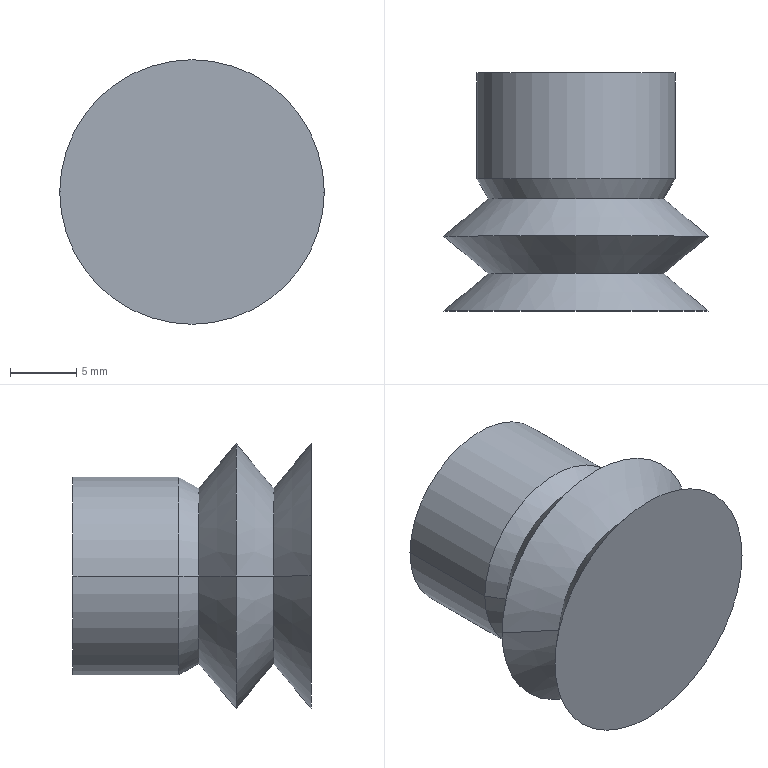Part | STEP file | JS2-20(0-19) | 1 solid | 18 faces | box 20 x 18 x 20 mm | volume 3384 mm3 | cone 8 | cylinder 6 | plane 4 | commonest cylinder face diameters 5 x2 7 x2 15 x2
STEP:
#1=CARTESIAN_POINT('',(0.,0.,0.));
#2=DIRECTION('',(0.,0.,1.));
#3=DIRECTION('',(1.,0.,0.));
#4=AXIS2_PLACEMENT_3D('',#1,#2,#3);
#5=CARTESIAN_POINT('',(-3.5,13.,0.));
#6=VERTEX_POINT('',#5);
#7=CARTESIAN_POINT('',(-3.5,15.,0.));
#8=VERTEX_POINT('',#7);
#9=CARTESIAN_POINT('',(-3.5,13.,0.));
#10=DIRECTION('',(0.,1.,0.));
#11=VECTOR('',#10,1.);
#12=LINE('',#9,#11);
#13=CARTESIAN_POINT('',(0.,13.,0.));
#14=DIRECTION('',(0.,1.,0.));
#15=DIRECTION('',(-1.,0.,0.));
#16=AXIS2_PLACEMENT_3D('',#13,#14,#15);
#17=CYLINDRICAL_SURFACE('',#16,3.5);
#18=CARTESIAN_POINT('',(6.283,0.));
#19=DIRECTION('',(0.,1.));
#20=VECTOR('',#19,1.);
#21=LINE('',#18,#20);
#22=(GEOMETRIC_REPRESENTATION_CONTEXT(2)PARAMETRIC_REPRESENTATION_CONTEXT()REPRESENTATION_CONTEXT('',''));
#23=DEFINITIONAL_REPRESENTATION('',(#21),#22);
#24=PCURVE('',#17,#23);
#25=CARTESIAN_POINT('',(0.,13.,0.));
#26=DIRECTION('',(0.,1.,0.));
#27=DIRECTION('',(-1.,0.,0.));
#28=AXIS2_PLACEMENT_3D('',#25,#26,#27);
#29=CYLINDRICAL_SURFACE('',#28,3.5);
#30=CARTESIAN_POINT('',(0.,0.));
#31=DIRECTION('',(0.,1.));
#32=VECTOR('',#31,1.);
#33=LINE('',#30,#32);
#34=(GEOMETRIC_REPRESENTATION_CONTEXT(2)PARAMETRIC_REPRESENTATION_CONTEXT()REPRESENTATION_CONTEXT('',''));
#35=DEFINITIONAL_REPRESENTATION('',(#33),#34);
#36=PCURVE('',#29,#35);
#37=SURFACE_CURVE('',#12,(#24,#36),.PCURVE_S1.);
#38=EDGE_CURVE('',#6,#8,#37,.T.);
#39=ORIENTED_EDGE('',*,*,#38,.T.);
#40=CARTESIAN_POINT('',(3.5,15.,0.));
#41=VERTEX_POINT('',#40);
#42=CARTESIAN_POINT('',(0.,15.,0.));
#43=DIRECTION('',(0.,1.,0.));
#44=DIRECTION('',(-1.,0.,0.));
#45=AXIS2_PLACEMENT_3D('',#42,#43,#44);
#46=CIRCLE('',#45,3.5);
#47=CARTESIAN_POINT('',(0.,2.));
#48=DIRECTION('',(1.,0.));
#49=VECTOR('',#48,1.);
#50=LINE('',#47,#49);
#51=(GEOMETRIC_REPRESENTATION_CONTEXT(2)PARAMETRIC_REPRESENTATION_CONTEXT()REPRESENTATION_CONTEXT('',''));
#52=DEFINITIONAL_REPRESENTATION('',(#50),#51);
#53=PCURVE('',#17,#52);
#54=CARTESIAN_POINT('',(0.,15.,0.));
#55=DIRECTION('',(0.,1.,0.));
#56=DIRECTION('',(-1.,0.,0.));
#57=AXIS2_PLACEMENT_3D('',#54,#55,#56);
#58=PLANE('',#57);
#59=CARTESIAN_POINT('',(0.,0.));
#60=DIRECTION('',(1.,0.));
#61=AXIS2_PLACEMENT_2D('',#59,#60);
#62=CIRCLE('',#61,3.5);
#63=(GEOMETRIC_REPRESENTATION_CONTEXT(2)PARAMETRIC_REPRESENTATION_CONTEXT()REPRESENTATION_CONTEXT('',''));
#64=DEFINITIONAL_REPRESENTATION('',(#62),#63);
#65=PCURVE('',#58,#64);
#66=SURFACE_CURVE('',#46,(#53,#65),.PCURVE_S1.);
#67=EDGE_CURVE('',#41,#8,#66,.T.);
#68=ORIENTED_EDGE('',*,*,#67,.F.);
#69=CARTESIAN_POINT('',(3.5,13.,0.));
#70=VERTEX_POINT('',#69);
#71=CARTESIAN_POINT('',(3.5,13.,0.));
#72=DIRECTION('',(0.,1.,0.));
#73=VECTOR('',#72,1.);
#74=LINE('',#71,#73);
#75=CARTESIAN_POINT('',(3.142,0.));
#76=DIRECTION('',(0.,1.));
#77=VECTOR('',#76,1.);
#78=LINE('',#75,#77);
#79=(GEOMETRIC_REPRESENTATION_CONTEXT(2)PARAMETRIC_REPRESENTATION_CONTEXT()REPRESENTATION_CONTEXT('',''));
#80=DEFINITIONAL_REPRESENTATION('',(#78),#79);
#81=PCURVE('',#17,#80);
#82=CARTESIAN_POINT('',(3.142,0.));
#83=DIRECTION('',(0.,1.));
#84=VECTOR('',#83,1.);
#85=LINE('',#82,#84);
#86=(GEOMETRIC_REPRESENTATION_CONTEXT(2)PARAMETRIC_REPRESENTATION_CONTEXT()REPRESENTATION_CONTEXT('',''));
#87=DEFINITIONAL_REPRESENTATION('',(#85),#86);
#88=PCURVE('',#29,#87);
#89=SURFACE_CURVE('',#74,(#81,#88),.PCURVE_S1.);
#90=EDGE_CURVE('',#70,#41,#89,.T.);
#91=ORIENTED_EDGE('',*,*,#90,.F.);
#92=CARTESIAN_POINT('',(0.,13.,0.));
#93=DIRECTION('',(0.,1.,0.));
#94=DIRECTION('',(-1.,0.,0.));
#95=AXIS2_PLACEMENT_3D('',#92,#93,#94);
#96=CIRCLE('',#95,3.5);
#97=CARTESIAN_POINT('',(0.,0.));
#98=DIRECTION('',(1.,0.));
#99=VECTOR('',#98,1.);
#100=LINE('',#97,#99);
#101=(GEOMETRIC_REPRESENTATION_CONTEXT(2)PARAMETRIC_REPRESENTATION_CONTEXT()REPRESENTATION_CONTEXT('',''));
#102=DEFINITIONAL_REPRESENTATION('',(#100),#101);
#103=PCURVE('',#17,#102);
#104=CARTESIAN_POINT('',(0.,13.,0.));
#105=DIRECTION('',(0.,1.,0.));
#106=DIRECTION('',(-1.,0.,0.));
#107=AXIS2_PLACEMENT_3D('',#104,#105,#106);
#108=PLANE('',#107);
#109=CARTESIAN_POINT('',(0.,0.));
#110=DIRECTION('',(1.,0.));
#111=AXIS2_PLACEMENT_2D('',#109,#110);
#112=CIRCLE('',#111,3.5);
#113=(GEOMETRIC_REPRESENTATION_CONTEXT(2)PARAMETRIC_REPRESENTATION_CONTEXT()REPRESENTATION_CONTEXT('',''));
#114=DEFINITIONAL_REPRESENTATION('',(#112),#113);
#115=PCURVE('',#108,#114);
#116=SURFACE_CURVE('',#96,(#103,#115),.PCURVE_S1.);
#117=EDGE_CURVE('',#70,#6,#116,.T.);
#118=ORIENTED_EDGE('',*,*,#117,.T.);
#119=EDGE_LOOP('',(#39,#68,#91,#118));
#120=FACE_BOUND('',#119,.F.);
#121=ADVANCED_FACE('',(#120),#17,.F.);
#122=CARTESIAN_POINT('',(-2.5,15.,0.));
#123=VERTEX_POINT('',#122);
#124=CARTESIAN_POINT('',(-2.5,18.,0.));
#125=VERTEX_POINT('',#124);
#126=CARTESIAN_POINT('',(-2.5,13.,0.));
#127=DIRECTION('',(0.,1.,0.));
#128=VECTOR('',#127,1.);
#129=LINE('',#126,#128);
#130=CARTESIAN_POINT('',(0.,13.,0.));
#131=DIRECTION('',(0.,1.,0.));
#132=DIRECTION('',(-1.,0.,0.));
#133=AXIS2_PLACEMENT_3D('',#130,#131,#132);
#134=CYLINDRICAL_SURFACE('',#133,2.5);
#135=CARTESIAN_POINT('',(6.283,0.));
#136=DIRECTION('',(0.,1.));
#137=VECTOR('',#136,1.);
#138=LINE('',#135,#137);
#139=(GEOMETRIC_REPRESENTATION_CONTEXT(2)PARAMETRIC_REPRESENTATION_CONTEXT()REPRESENTATION_CONTEXT('',''));
#140=DEFINITIONAL_REPRESENTATION('',(#138),#139);
#141=PCURVE('',#134,#140);
#142=CARTESIAN_POINT('',(0.,13.,0.));
#143=DIRECTION('',(0.,1.,0.));
#144=DIRECTION('',(-1.,0.,0.));
#145=AXIS2_PLACEMENT_3D('',#142,#143,#144);
#146=CYLINDRICAL_SURFACE('',#145,2.5);
#147=CARTESIAN_POINT('',(0.,0.));
#148=DIRECTION('',(0.,1.));
#149=VECTOR('',#148,1.);
#150=LINE('',#147,#149);
#151=(GEOMETRIC_REPRESENTATION_CONTEXT(2)PARAMETRIC_REPRESENTATION_CONTEXT()REPRESENTATION_CONTEXT('',''));
#152=DEFINITIONAL_REPRESENTATION('',(#150),#151);
#153=PCURVE('',#146,#152);
#154=SURFACE_CURVE('',#129,(#141,#153),.PCURVE_S1.);
#155=EDGE_CURVE('',#123,#125,#154,.T.);
#156=ORIENTED_EDGE('',*,*,#155,.T.);
#157=CARTESIAN_POINT('',(2.5,18.,0.));
#158=VERTEX_POINT('',#157);
#159=CARTESIAN_POINT('',(0.,18.,0.));
#160=DIRECTION('',(0.,1.,0.));
#161=DIRECTION('',(-1.,0.,0.));
#162=AXIS2_PLACEMENT_3D('',#159,#160,#161);
#163=CIRCLE('',#162,2.5);
#164=CARTESIAN_POINT('',(0.,5.));
#165=DIRECTION('',(1.,0.));
#166=VECTOR('',#165,1.);
#167=LINE('',#164,#166);
#168=(GEOMETRIC_REPRESENTATION_CONTEXT(2)PARAMETRIC_REPRESENTATION_CONTEXT()REPRESENTATION_CONTEXT('',''));
#169=DEFINITIONAL_REPRESENTATION('',(#167),#168);
#170=PCURVE('',#134,#169);
#171=CARTESIAN_POINT('',(-7.5,18.,0.));
#172=DIRECTION('',(0.,1.,0.));
#173=DIRECTION('',(-1.,0.,0.));
#174=AXIS2_PLACEMENT_3D('',#171,#172,#173);
#175=PLANE('',#174);
#176=CARTESIAN_POINT('',(-7.5,0.));
#177=DIRECTION('',(1.,0.));
#178=AXIS2_PLACEMENT_2D('',#176,#177);
#179=CIRCLE('',#178,2.5);
#180=(GEOMETRIC_REPRESENTATION_CONTEXT(2)PARAMETRIC_REPRESENTATION_CONTEXT()REPRESENTATION_CONTEXT('',''));
#181=DEFINITIONAL_REPRESENTATION('',(#179),#180);
#182=PCURVE('',#175,#181);
#183=SURFACE_CURVE('',#163,(#170,#182),.PCURVE_S1.);
#184=EDGE_CURVE('',#158,#125,#183,.T.);
#185=ORIENTED_EDGE('',*,*,#184,.F.);
#186=CARTESIAN_POINT('',(2.5,15.,0.));
#187=VERTEX_POINT('',#186);
#188=CARTESIAN_POINT('',(2.5,13.,0.));
#189=DIRECTION('',(0.,1.,0.));
#190=VECTOR('',#189,1.);
#191=LINE('',#188,#190);
#192=CARTESIAN_POINT('',(3.142,0.));
#193=DIRECTION('',(0.,1.));
#194=VECTOR('',#193,1.);
#195=LINE('',#192,#194);
#196=(GEOMETRIC_REPRESENTATION_CONTEXT(2)PARAMETRIC_REPRESENTATION_CONTEXT()REPRESENTATION_CONTEXT('',''));
#197=DEFINITIONAL_REPRESENTATION('',(#195),#196);
#198=PCURVE('',#134,#197);
#199=CARTESIAN_POINT('',(3.142,0.));
#200=DIRECTION('',(0.,1.));
#201=VECTOR('',#200,1.);
#202=LINE('',#199,#201);
#203=(GEOMETRIC_REPRESENTATION_CONTEXT(2)PARAMETRIC_REPRESENTATION_CONTEXT()REPRESENTATION_CONTEXT('',''));
#204=DEFINITIONAL_REPRESENTATION('',(#202),#203);
#205=PCURVE('',#146,#204);
#206=SURFACE_CURVE('',#191,(#198,#205),.PCURVE_S1.);
#207=EDGE_CURVE('',#187,#158,#206,.T.);
#208=ORIENTED_EDGE('',*,*,#207,.F.);
#209=CARTESIAN_POINT('',(0.,15.,0.));
#210=DIRECTION('',(0.,-1.,0.));
#211=DIRECTION('',(-1.,0.,0.));
#212=AXIS2_PLACEMENT_3D('',#209,#210,#211);
#213=CIRCLE('',#212,2.5);
#214=CARTESIAN_POINT('',(6.283,2.));
#215=DIRECTION('',(-1.,0.));
#216=VECTOR('',#215,1.);
#217=LINE('',#214,#216);
#218=(GEOMETRIC_REPRESENTATION_CONTEXT(2)PARAMETRIC_REPRESENTATION_CONTEXT()REPRESENTATION_CONTEXT('',''));
#219=DEFINITIONAL_REPRESENTATION('',(#217),#218);
#220=PCURVE('',#134,#219);
#221=CARTESIAN_POINT('',(2.5,0.));
#222=CARTESIAN_POINT('',(2.5,-4.33));
#223=CARTESIAN_POINT('',(-1.25,-2.165));
#224=CARTESIAN_POINT('',(-5.,0.));
#225=CARTESIAN_POINT('',(-1.25,2.165));
#226=CARTESIAN_POINT('',(2.5,4.33));
#227=CARTESIAN_POINT('',(2.5,0.));
#228=(BOUNDED_CURVE()B_SPLINE_CURVE(2,(#221,#222,#223,#224,#225,#226,#227),.UNSPECIFIED.,.T.,.F.)B_SPLINE_CURVE_WITH_KNOTS((1,2,2,2,2,1),(-2.094,0.,2.094,4.189,6.283,8.378),.UNSPECIFIED.)CURVE()GEOMETRIC_REPRESENTATION_ITEM()RATIONAL_B_SPLINE_CURVE((1.,0.5,1.,0.5,1.,0.5,1.))REPRESENTATION_ITEM(''));
#229=(GEOMETRIC_REPRESENTATION_CONTEXT(2)PARAMETRIC_REPRESENTATION_CONTEXT()REPRESENTATION_CONTEXT('',''));
#230=DEFINITIONAL_REPRESENTATION('',(#228),#229);
#231=PCURVE('',#58,#230);
#232=SURFACE_CURVE('',#213,(#220,#231),.PCURVE_S1.);
#233=EDGE_CURVE('',#123,#187,#232,.T.);
#234=ORIENTED_EDGE('',*,*,#233,.F.);
#235=EDGE_LOOP('',(#156,#185,#208,#234));
#236=FACE_BOUND('',#235,.F.);
#237=ADVANCED_FACE('',(#236),#134,.F.);
#238=CARTESIAN_POINT('',(-7.5,10.,0.));
#239=VERTEX_POINT('',#238);
#240=CARTESIAN_POINT('',(7.5,10.,0.));
#241=VERTEX_POINT('',#240);
#242=CARTESIAN_POINT('',(0.,10.,0.));
#243=DIRECTION('',(0.,1.,0.));
#244=DIRECTION('',(-1.,0.,0.));
#245=AXIS2_PLACEMENT_3D('',#242,#243,#244);
#246=CIRCLE('',#245,7.5);
#247=CARTESIAN_POINT('',(0.,18.,0.));
#248=DIRECTION('',(0.,1.,0.));
#249=DIRECTION('',(-1.,0.,0.));
#250=AXIS2_PLACEMENT_3D('',#247,#248,#249);
#251=CYLINDRICAL_SURFACE('',#250,7.5);
#252=CARTESIAN_POINT('',(0.,-8.));
#253=DIRECTION('',(1.,0.));
#254=VECTOR('',#253,1.);
#255=LINE('',#252,#254);
#256=(GEOMETRIC_REPRESENTATION_CONTEXT(2)PARAMETRIC_REPRESENTATION_CONTEXT()REPRESENTATION_CONTEXT('',''));
#257=DEFINITIONAL_REPRESENTATION('',(#255),#256);
#258=PCURVE('',#251,#257);
#259=CARTESIAN_POINT('',(0.,10.,0.));
#260=DIRECTION('',(0.,1.,0.));
#261=DIRECTION('',(-1.,0.,0.));
#262=AXIS2_PLACEMENT_3D('',#259,#260,#261);
#263=CONICAL_SURFACE('',#262,7.5,0.5236);
#264=CARTESIAN_POINT('',(0.,0.));
#265=DIRECTION('',(1.,0.));
#266=VECTOR('',#265,1.);
#267=LINE('',#264,#266);
#268=(GEOMETRIC_REPRESENTATION_CONTEXT(2)PARAMETRIC_REPRESENTATION_CONTEXT()REPRESENTATION_CONTEXT('',''));
#269=DEFINITIONAL_REPRESENTATION('',(#267),#268);
#270=PCURVE('',#263,#269);
#271=SURFACE_CURVE('',#246,(#258,#270),.PCURVE_S1.);
#272=EDGE_CURVE('',#239,#241,#271,.T.);
#273=ORIENTED_EDGE('',*,*,#272,.T.);
#274=CARTESIAN_POINT('',(7.5,18.,0.));
#275=VERTEX_POINT('',#274);
#276=CARTESIAN_POINT('',(7.5,18.,0.));
#277=DIRECTION('',(0.,1.,0.));
#278=VECTOR('',#277,1.);
#279=LINE('',#276,#278);
#280=CARTESIAN_POINT('',(3.142,0.));
#281=DIRECTION('',(0.,1.));
#282=VECTOR('',#281,1.);
#283=LINE('',#280,#282);
#284=(GEOMETRIC_REPRESENTATION_CONTEXT(2)PARAMETRIC_REPRESENTATION_CONTEXT()REPRESENTATION_CONTEXT('',''));
#285=DEFINITIONAL_REPRESENTATION('',(#283),#284);
#286=PCURVE('',#251,#285);
#287=CARTESIAN_POINT('',(0.,18.,0.));
#288=DIRECTION('',(0.,1.,0.));
#289=DIRECTION('',(-1.,0.,0.));
#290=AXIS2_PLACEMENT_3D('',#287,#288,#289);
#291=CYLINDRICAL_SURFACE('',#290,7.5);
#292=CARTESIAN_POINT('',(3.142,0.));
#293=DIRECTION('',(0.,1.));
#294=VECTOR('',#293,1.);
#295=LINE('',#292,#294);
#296=(GEOMETRIC_REPRESENTATION_CONTEXT(2)PARAMETRIC_REPRESENTATION_CONTEXT()REPRESENTATION_CONTEXT('',''));
#297=DEFINITIONAL_REPRESENTATION('',(#295),#296);
#298=PCURVE('',#291,#297);
#299=SURFACE_CURVE('',#279,(#286,#298),.PCURVE_S1.);
#300=EDGE_CURVE('',#241,#275,#299,.T.);
#301=ORIENTED_EDGE('',*,*,#300,.T.);
#302=CARTESIAN_POINT('',(-7.5,18.,0.));
#303=VERTEX_POINT('',#302);
#304=CARTESIAN_POINT('',(0.,18.,0.));
#305=DIRECTION('',(0.,1.,0.));
#306=DIRECTION('',(-1.,0.,0.));
#307=AXIS2_PLACEMENT_3D('',#304,#305,#306);
#308=CIRCLE('',#307,7.5);
#309=CARTESIAN_POINT('',(0.,0.));
#310=DIRECTION('',(1.,0.));
#311=VECTOR('',#310,1.);
#312=LINE('',#309,#311);
#313=(GEOMETRIC_REPRESENTATION_CONTEXT(2)PARAMETRIC_REPRESENTATION_CONTEXT()REPRESENTATION_CONTEXT('',''));
#314=DEFINITIONAL_REPRESENTATION('',(#312),#313);
#315=PCURVE('',#251,#314);
#316=CARTESIAN_POINT('',(-7.5,0.));
#317=DIRECTION('',(1.,0.));
#318=AXIS2_PLACEMENT_2D('',#316,#317);
#319=CIRCLE('',#318,7.5);
#320=(GEOMETRIC_REPRESENTATION_CONTEXT(2)PARAMETRIC_REPRESENTATION_CONTEXT()REPRESENTATION_CONTEXT('',''));
#321=DEFINITIONAL_REPRESENTATION('',(#319),#320);
#322=PCURVE('',#175,#321);
#323=SURFACE_CURVE('',#308,(#315,#322),.PCURVE_S1.);
#324=EDGE_CURVE('',#303,#275,#323,.T.);
#325=ORIENTED_EDGE('',*,*,#324,.F.);
#326=CARTESIAN_POINT('',(-7.5,18.,0.));
#327=DIRECTION('',(0.,1.,0.));
#328=VECTOR('',#327,1.);
#329=LINE('',#326,#328);
#330=CARTESIAN_POINT('',(0.,0.));
#331=DIRECTION('',(0.,1.));
#332=VECTOR('',#331,1.);
#333=LINE('',#330,#332);
#334=(GEOMETRIC_REPRESENTATION_CONTEXT(2)PARAMETRIC_REPRESENTATION_CONTEXT()REPRESENTATION_CONTEXT('',''));
#335=DEFINITIONAL_REPRESENTATION('',(#333),#334);
#336=PCURVE('',#251,#335);
#337=CARTESIAN_POINT('',(6.283,0.));
#338=DIRECTION('',(0.,1.));
#339=VECTOR('',#338,1.);
#340=LINE('',#337,#339);
#341=(GEOMETRIC_REPRESENTATION_CONTEXT(2)PARAMETRIC_REPRESENTATION_CONTEXT()REPRESENTATION_CONTEXT('',''));
#342=DEFINITIONAL_REPRESENTATION('',(#340),#341);
#343=PCURVE('',#291,#342);
#344=SURFACE_CURVE('',#329,(#336,#343),.PCURVE_S1.);
#345=EDGE_CURVE('',#239,#303,#344,.T.);
#346=ORIENTED_EDGE('',*,*,#345,.F.);
#347=EDGE_LOOP('',(#273,#301,#325,#346));
#348=FACE_BOUND('',#347,.T.);
#349=ADVANCED_FACE('',(#348),#251,.T.);
#350=CARTESIAN_POINT('',(-6.628,8.489,0.));
#351=VERTEX_POINT('',#350);
#352=CARTESIAN_POINT('',(6.628,8.489,0.));
#353=VERTEX_POINT('',#352);
#354=CARTESIAN_POINT('',(0.,8.489,0.));
#355=DIRECTION('',(0.,1.,0.));
#356=DIRECTION('',(-1.,0.,0.));
#357=AXIS2_PLACEMENT_3D('',#354,#355,#356);
#358=CIRCLE('',#357,6.628);
#359=CARTESIAN_POINT('',(0.,-1.511));
#360=DIRECTION('',(1.,0.));
#361=VECTOR('',#360,1.);
#362=LINE('',#359,#361);
#363=(GEOMETRIC_REPRESENTATION_CONTEXT(2)PARAMETRIC_REPRESENTATION_CONTEXT()REPRESENTATION_CONTEXT('',''));
#364=DEFINITIONAL_REPRESENTATION('',(#362),#363);
#365=PCURVE('',#263,#364);
#366=CARTESIAN_POINT('',(0.,8.489,0.));
#367=DIRECTION('',(0.,-1.,0.));
#368=DIRECTION('',(1.,0.,0.));
#369=AXIS2_PLACEMENT_3D('',#366,#367,#368);
#370=CONICAL_SURFACE('',#369,6.628,0.8727);
#371=CARTESIAN_POINT('',(3.142,0.));
#372=DIRECTION('',(-1.,0.));
#373=VECTOR('',#372,1.);
#374=LINE('',#371,#373);
#375=(GEOMETRIC_REPRESENTATION_CONTEXT(2)PARAMETRIC_REPRESENTATION_CONTEXT()REPRESENTATION_CONTEXT('',''));
#376=DEFINITIONAL_REPRESENTATION('',(#374),#375);
#377=PCURVE('',#370,#376);
#378=SURFACE_CURVE('',#358,(#365,#377),.PCURVE_S1.);
#379=EDGE_CURVE('',#351,#353,#378,.T.);
#380=ORIENTED_EDGE('',*,*,#379,.T.);
#381=CARTESIAN_POINT('',(7.5,10.,0.));
#382=DIRECTION('',(0.5,0.866,0.));
#383=VECTOR('',#382,1.);
#384=LINE('',#381,#383);
#385=CARTESIAN_POINT('',(3.142,0.));
#386=DIRECTION('',(0.,1.));
#387=VECTOR('',#386,1.);
#388=LINE('',#385,#387);
#389=(GEOMETRIC_REPRESENTATION_CONTEXT(2)PARAMETRIC_REPRESENTATION_CONTEXT()REPRESENTATION_CONTEXT('',''));
#390=DEFINITIONAL_REPRESENTATION('',(#388),#389);
#391=PCURVE('',#263,#390);
#392=CARTESIAN_POINT('',(0.,10.,0.));
#393=DIRECTION('',(0.,1.,0.));
#394=DIRECTION('',(-1.,0.,0.));
#395=AXIS2_PLACEMENT_3D('',#392,#393,#394);
#396=CONICAL_SURFACE('',#395,7.5,0.5236);
#397=CARTESIAN_POINT('',(3.142,0.));
#398=DIRECTION('',(0.,1.));
#399=VECTOR('',#398,1.);
#400=LINE('',#397,#399);
#401=(GEOMETRIC_REPRESENTATION_CONTEXT(2)PARAMETRIC_REPRESENTATION_CONTEXT()REPRESENTATION_CONTEXT('',''));
#402=DEFINITIONAL_REPRESENTATION('',(#400),#401);
#403=PCURVE('',#396,#402);
#404=SURFACE_CURVE('',#384,(#391,#403),.PCURVE_S1.);
#405=EDGE_CURVE('',#353,#241,#404,.T.);
#406=ORIENTED_EDGE('',*,*,#405,.T.);
#407=ORIENTED_EDGE('',*,*,#272,.F.);
#408=CARTESIAN_POINT('',(-7.5,10.,0.));
#409=DIRECTION('',(-0.5,0.866,0.));
#410=VECTOR('',#409,1.);
#411=LINE('',#408,#410);
#412=CARTESIAN_POINT('',(0.,0.));
#413=DIRECTION('',(0.,1.));
#414=VECTOR('',#413,1.);
#415=LINE('',#412,#414);
#416=(GEOMETRIC_REPRESENTATION_CONTEXT(2)PARAMETRIC_REPRESENTATION_CONTEXT()REPRESENTATION_CONTEXT('',''));
#417=DEFINITIONAL_REPRESENTATION('',(#415),#416);
#418=PCURVE('',#263,#417);
#419=CARTESIAN_POINT('',(6.283,0.));
#420=DIRECTION('',(0.,1.));
#421=VECTOR('',#420,1.);
#422=LINE('',#419,#421);
#423=(GEOMETRIC_REPRESENTATION_CONTEXT(2)PARAMETRIC_REPRESENTATION_CONTEXT()REPRESENTATION_CONTEXT('',''));
#424=DEFINITIONAL_REPRESENTATION('',(#422),#423);
#425=PCURVE('',#396,#424);
#426=SURFACE_CURVE('',#411,(#418,#425),.PCURVE_S1.);
#427=EDGE_CURVE('',#351,#239,#426,.T.);
#428=ORIENTED_EDGE('',*,*,#427,.F.);
#429=EDGE_LOOP('',(#380,#406,#407,#428));
#430=FACE_BOUND('',#429,.T.);
#431=ADVANCED_FACE('',(#430),#263,.T.);
#432=ORIENTED_EDGE('',*,*,#379,.F.);
#433=CARTESIAN_POINT('',(-10.,5.659,0.));
#434=VERTEX_POINT('',#433);
#435=CARTESIAN_POINT('',(-6.628,8.489,0.));
#436=DIRECTION('',(-0.766,-0.6428,0.));
#437=VECTOR('',#436,1.);
#438=LINE('',#435,#437);
#439=CARTESIAN_POINT('',(3.142,0.));
#440=DIRECTION('',(0.,1.));
#441=VECTOR('',#440,1.);
#442=LINE('',#439,#441);
#443=(GEOMETRIC_REPRESENTATION_CONTEXT(2)PARAMETRIC_REPRESENTATION_CONTEXT()REPRESENTATION_CONTEXT('',''));
#444=DEFINITIONAL_REPRESENTATION('',(#442),#443);
#445=PCURVE('',#370,#444);
#446=CARTESIAN_POINT('',(0.,8.489,0.));
#447=DIRECTION('',(0.,-1.,0.));
#448=DIRECTION('',(1.,0.,0.));
#449=AXIS2_PLACEMENT_3D('',#446,#447,#448);
#450=CONICAL_SURFACE('',#449,6.628,0.8727);
#451=CARTESIAN_POINT('',(3.142,0.));
#452=DIRECTION('',(0.,1.));
#453=VECTOR('',#452,1.);
#454=LINE('',#451,#453);
#455=(GEOMETRIC_REPRESENTATION_CONTEXT(2)PARAMETRIC_REPRESENTATION_CONTEXT()REPRESENTATION_CONTEXT('',''));
#456=DEFINITIONAL_REPRESENTATION('',(#454),#455);
#457=PCURVE('',#450,#456);
#458=SURFACE_CURVE('',#438,(#445,#457),.PCURVE_S1.);
#459=EDGE_CURVE('',#351,#434,#458,.T.);
#460=ORIENTED_EDGE('',*,*,#459,.T.);
#461=CARTESIAN_POINT('',(10.,5.659,0.));
#462=VERTEX_POINT('',#461);
#463=CARTESIAN_POINT('',(0.,5.659,0.));
#464=DIRECTION('',(0.,1.,0.));
#465=DIRECTION('',(-1.,0.,0.));
#466=AXIS2_PLACEMENT_3D('',#463,#464,#465);
#467=CIRCLE('',#466,10.);
#468=CARTESIAN_POINT('',(3.142,2.83));
#469=DIRECTION('',(-1.,0.));
#470=VECTOR('',#469,1.);
#471=LINE('',#468,#470);
#472=(GEOMETRIC_REPRESENTATION_CONTEXT(2)PARAMETRIC_REPRESENTATION_CONTEXT()REPRESENTATION_CONTEXT('',''));
#473=DEFINITIONAL_REPRESENTATION('',(#471),#472);
#474=PCURVE('',#370,#473);
#475=CARTESIAN_POINT('',(0.,5.659,0.));
#476=DIRECTION('',(0.,1.,0.));
#477=DIRECTION('',(-1.,0.,0.));
#478=AXIS2_PLACEMENT_3D('',#475,#476,#477);
#479=CONICAL_SURFACE('',#478,10.,0.8727);
#480=CARTESIAN_POINT('',(0.,0.));
#481=DIRECTION('',(1.,0.));
#482=VECTOR('',#481,1.);
#483=LINE('',#480,#482);
#484=(GEOMETRIC_REPRESENTATION_CONTEXT(2)PARAMETRIC_REPRESENTATION_CONTEXT()REPRESENTATION_CONTEXT('',''));
#485=DEFINITIONAL_REPRESENTATION('',(#483),#484);
#486=PCURVE('',#479,#485);
#487=SURFACE_CURVE('',#467,(#474,#486),.PCURVE_S1.);
#488=EDGE_CURVE('',#434,#462,#487,.T.);
#489=ORIENTED_EDGE('',*,*,#488,.T.);
#490=CARTESIAN_POINT('',(6.628,8.489,0.));
#491=DIRECTION('',(0.766,-0.6428,0.));
#492=VECTOR('',#491,1.);
#493=LINE('',#490,#492);
#494=CARTESIAN_POINT('',(0.,0.));
#495=DIRECTION('',(0.,1.));
#496=VECTOR('',#495,1.);
#497=LINE('',#494,#496);
#498=(GEOMETRIC_REPRESENTATION_CONTEXT(2)PARAMETRIC_REPRESENTATION_CONTEXT()REPRESENTATION_CONTEXT('',''));
#499=DEFINITIONAL_REPRESENTATION('',(#497),#498);
#500=PCURVE('',#370,#499);
#501=CARTESIAN_POINT('',(6.283,0.));
#502=DIRECTION('',(0.,1.));
#503=VECTOR('',#502,1.);
#504=LINE('',#501,#503);
#505=(GEOMETRIC_REPRESENTATION_CONTEXT(2)PARAMETRIC_REPRESENTATION_CONTEXT()REPRESENTATION_CONTEXT('',''));
#506=DEFINITIONAL_REPRESENTATION('',(#504),#505);
#507=PCURVE('',#450,#506);
#508=SURFACE_CURVE('',#493,(#500,#507),.PCURVE_S1.);
#509=EDGE_CURVE('',#353,#462,#508,.T.);
#510=ORIENTED_EDGE('',*,*,#509,.F.);
#511=EDGE_LOOP('',(#432,#460,#489,#510));
#512=FACE_BOUND('',#511,.T.);
#513=ADVANCED_FACE('',(#512),#370,.T.);
#514=CARTESIAN_POINT('',(-6.628,2.83,0.));
#515=VERTEX_POINT('',#514);
#516=CARTESIAN_POINT('',(6.628,2.83,0.));
#517=VERTEX_POINT('',#516);
#518=CARTESIAN_POINT('',(0.,2.83,0.));
#519=DIRECTION('',(0.,1.,0.));
#520=DIRECTION('',(-1.,0.,0.));
#521=AXIS2_PLACEMENT_3D('',#518,#519,#520);
#522=CIRCLE('',#521,6.628);
#523=CARTESIAN_POINT('',(0.,-2.83));
#524=DIRECTION('',(1.,0.));
#525=VECTOR('',#524,1.);
#526=LINE('',#523,#525);
#527=(GEOMETRIC_REPRESENTATION_CONTEXT(2)PARAMETRIC_REPRESENTATION_CONTEXT()REPRESENTATION_CONTEXT('',''));
#528=DEFINITIONAL_REPRESENTATION('',(#526),#527);
#529=PCURVE('',#479,#528);
#530=CARTESIAN_POINT('',(0.,2.83,0.));
#531=DIRECTION('',(0.,-1.,0.));
#532=DIRECTION('',(1.,0.,0.));
#533=AXIS2_PLACEMENT_3D('',#530,#531,#532);
#534=CONICAL_SURFACE('',#533,6.628,0.8727);
#535=CARTESIAN_POINT('',(3.142,0.));
#536=DIRECTION('',(-1.,0.));
#537=VECTOR('',#536,1.);
#538=LINE('',#535,#537);
#539=(GEOMETRIC_REPRESENTATION_CONTEXT(2)PARAMETRIC_REPRESENTATION_CONTEXT()REPRESENTATION_CONTEXT('',''));
#540=DEFINITIONAL_REPRESENTATION('',(#538),#539);
#541=PCURVE('',#534,#540);
#542=SURFACE_CURVE('',#522,(#529,#541),.PCURVE_S1.);
#543=EDGE_CURVE('',#515,#517,#542,.T.);
#544=ORIENTED_EDGE('',*,*,#543,.T.);
#545=CARTESIAN_POINT('',(10.,5.659,0.));
#546=DIRECTION('',(0.766,0.6428,0.));
#547=VECTOR('',#546,1.);
#548=LINE('',#545,#547);
#549=CARTESIAN_POINT('',(3.142,0.));
#550=DIRECTION('',(0.,1.));
#551=VECTOR('',#550,1.);
#552=LINE('',#549,#551);
#553=(GEOMETRIC_REPRESENTATION_CONTEXT(2)PARAMETRIC_REPRESENTATION_CONTEXT()REPRESENTATION_CONTEXT('',''));
#554=DEFINITIONAL_REPRESENTATION('',(#552),#553);
#555=PCURVE('',#479,#554);
#556=CARTESIAN_POINT('',(0.,5.659,0.));
#557=DIRECTION('',(0.,1.,0.));
#558=DIRECTION('',(-1.,0.,0.));
#559=AXIS2_PLACEMENT_3D('',#556,#557,#558);
#560=CONICAL_SURFACE('',#559,10.,0.8727);
#561=CARTESIAN_POINT('',(3.142,0.));
#562=DIRECTION('',(0.,1.));
#563=VECTOR('',#562,1.);
#564=LINE('',#561,#563);
#565=(GEOMETRIC_REPRESENTATION_CONTEXT(2)PARAMETRIC_REPRESENTATION_CONTEXT()REPRESENTATION_CONTEXT('',''));
#566=DEFINITIONAL_REPRESENTATION('',(#564),#565);
#567=PCURVE('',#560,#566);
#568=SURFACE_CURVE('',#548,(#555,#567),.PCURVE_S1.);
#569=EDGE_CURVE('',#517,#462,#568,.T.);
#570=ORIENTED_EDGE('',*,*,#569,.T.);
#571=ORIENTED_EDGE('',*,*,#488,.F.);
#572=CARTESIAN_POINT('',(-10.,5.659,0.));
#573=DIRECTION('',(-0.766,0.6428,0.));
#574=VECTOR('',#573,1.);
#575=LINE('',#572,#574);
#576=CARTESIAN_POINT('',(0.,0.));
#577=DIRECTION('',(0.,1.));
#578=VECTOR('',#577,1.);
#579=LINE('',#576,#578);
#580=(GEOMETRIC_REPRESENTATION_CONTEXT(2)PARAMETRIC_REPRESENTATION_CONTEXT()REPRESENTATION_CONTEXT('',''));
#581=DEFINITIONAL_REPRESENTATION('',(#579),#580);
#582=PCURVE('',#479,#581);
#583=CARTESIAN_POINT('',(6.283,0.));
#584=DIRECTION('',(0.,1.));
#585=VECTOR('',#584,1.);
#586=LINE('',#583,#585);
#587=(GEOMETRIC_REPRESENTATION_CONTEXT(2)PARAMETRIC_REPRESENTATION_CONTEXT()REPRESENTATION_CONTEXT('',''));
#588=DEFINITIONAL_REPRESENTATION('',(#586),#587);
#589=PCURVE('',#560,#588);
#590=SURFACE_CURVE('',#575,(#582,#589),.PCURVE_S1.);
#591=EDGE_CURVE('',#515,#434,#590,.T.);
#592=ORIENTED_EDGE('',*,*,#591,.F.);
#593=EDGE_LOOP('',(#544,#570,#571,#592));
#594=FACE_BOUND('',#593,.T.);
#595=ADVANCED_FACE('',(#594),#479,.T.);
#596=ORIENTED_EDGE('',*,*,#543,.F.);
#597=CARTESIAN_POINT('',(-10.,0.,0.));
#598=VERTEX_POINT('',#597);
#599=CARTESIAN_POINT('',(-6.628,2.83,0.));
#600=DIRECTION('',(-0.766,-0.6428,0.));
#601=VECTOR('',#600,1.);
#602=LINE('',#599,#601);
#603=CARTESIAN_POINT('',(3.142,0.));
#604=DIRECTION('',(0.,1.));
#605=VECTOR('',#604,1.);
#606=LINE('',#603,#605);
#607=(GEOMETRIC_REPRESENTATION_CONTEXT(2)PARAMETRIC_REPRESENTATION_CONTEXT()REPRESENTATION_CONTEXT('',''));
#608=DEFINITIONAL_REPRESENTATION('',(#606),#607);
#609=PCURVE('',#534,#608);
#610=CARTESIAN_POINT('',(0.,2.83,0.));
#611=DIRECTION('',(0.,-1.,0.));
#612=DIRECTION('',(1.,0.,0.));
#613=AXIS2_PLACEMENT_3D('',#610,#611,#612);
#614=CONICAL_SURFACE('',#613,6.628,0.8727);
#615=CARTESIAN_POINT('',(3.142,0.));
#616=DIRECTION('',(0.,1.));
#617=VECTOR('',#616,1.);
#618=LINE('',#615,#617);
#619=(GEOMETRIC_REPRESENTATION_CONTEXT(2)PARAMETRIC_REPRESENTATION_CONTEXT()REPRESENTATION_CONTEXT('',''));
#620=DEFINITIONAL_REPRESENTATION('',(#618),#619);
#621=PCURVE('',#614,#620);
#622=SURFACE_CURVE('',#602,(#609,#621),.PCURVE_S1.);
#623=EDGE_CURVE('',#515,#598,#622,.T.);
#624=ORIENTED_EDGE('',*,*,#623,.T.);
#625=CARTESIAN_POINT('',(10.,0.,0.));
#626=VERTEX_POINT('',#625);
#627=CARTESIAN_POINT('',(0.,0.,0.));
#628=DIRECTION('',(0.,1.,0.));
#629=DIRECTION('',(-1.,0.,0.));
#630=AXIS2_PLACEMENT_3D('',#627,#628,#629);
#631=CIRCLE('',#630,10.);
#632=CARTESIAN_POINT('',(3.142,2.83));
#633=DIRECTION('',(-1.,0.));
#634=VECTOR('',#633,1.);
#635=LINE('',#632,#634);
#636=(GEOMETRIC_REPRESENTATION_CONTEXT(2)PARAMETRIC_REPRESENTATION_CONTEXT()REPRESENTATION_CONTEXT('',''));
#637=DEFINITIONAL_REPRESENTATION('',(#635),#636);
#638=PCURVE('',#534,#637);
#639=CARTESIAN_POINT('',(0.,0.,0.));
#640=DIRECTION('',(0.,-1.,0.));
#641=DIRECTION('',(1.,0.,0.));
#642=AXIS2_PLACEMENT_3D('',#639,#640,#641);
#643=PLANE('',#642);
#644=CARTESIAN_POINT('',(-10.,0.));
#645=CARTESIAN_POINT('',(-10.,17.321));
#646=CARTESIAN_POINT('',(5.,8.66));
#647=CARTESIAN_POINT('',(20.,0.));
#648=CARTESIAN_POINT('',(5.,-8.66));
#649=CARTESIAN_POINT('',(-10.,-17.321));
#650=CARTESIAN_POINT('',(-10.,0.));
#651=(BOUNDED_CURVE()B_SPLINE_CURVE(2,(#644,#645,#646,#647,#648,#649,#650),.UNSPECIFIED.,.T.,.F.)B_SPLINE_CURVE_WITH_KNOTS((1,2,2,2,2,1),(-2.094,0.,2.094,4.189,6.283,8.378),.UNSPECIFIED.)CURVE()GEOMETRIC_REPRESENTATION_ITEM()RATIONAL_B_SPLINE_CURVE((1.,0.5,1.,0.5,1.,0.5,1.))REPRESENTATION_ITEM(''));
#652=(GEOMETRIC_REPRESENTATION_CONTEXT(2)PARAMETRIC_REPRESENTATION_CONTEXT()REPRESENTATION_CONTEXT('',''));
#653=DEFINITIONAL_REPRESENTATION('',(#651),#652);
#654=PCURVE('',#643,#653);
#655=SURFACE_CURVE('',#631,(#638,#654),.PCURVE_S1.);
#656=EDGE_CURVE('',#598,#626,#655,.T.);
#657=ORIENTED_EDGE('',*,*,#656,.T.);
#658=CARTESIAN_POINT('',(6.628,2.83,0.));
#659=DIRECTION('',(0.766,-0.6428,0.));
#660=VECTOR('',#659,1.);
#661=LINE('',#658,#660);
#662=CARTESIAN_POINT('',(0.,0.));
#663=DIRECTION('',(0.,1.));
#664=VECTOR('',#663,1.);
#665=LINE('',#662,#664);
#666=(GEOMETRIC_REPRESENTATION_CONTEXT(2)PARAMETRIC_REPRESENTATION_CONTEXT()REPRESENTATION_CONTEXT('',''));
#667=DEFINITIONAL_REPRESENTATION('',(#665),#666);
#668=PCURVE('',#534,#667);
#669=CARTESIAN_POINT('',(6.283,0.));
#670=DIRECTION('',(0.,1.));
#671=VECTOR('',#670,1.);
#672=LINE('',#669,#671);
#673=(GEOMETRIC_REPRESENTATION_CONTEXT(2)PARAMETRIC_REPRESENTATION_CONTEXT()REPRESENTATION_CONTEXT('',''));
#674=DEFINITIONAL_REPRESENTATION('',(#672),#673);
#675=PCURVE('',#614,#674);
#676=SURFACE_CURVE('',#661,(#668,#675),.PCURVE_S1.);
#677=EDGE_CURVE('',#517,#626,#676,.T.);
#678=ORIENTED_EDGE('',*,*,#677,.F.);
#679=EDGE_LOOP('',(#596,#624,#657,#678));
#680=FACE_BOUND('',#679,.T.);
#681=ADVANCED_FACE('',(#680),#534,.T.);
#682=CARTESIAN_POINT('',(0.,0.,0.));
#683=DIRECTION('',(0.,1.,0.));
#684=DIRECTION('',(-1.,0.,0.));
#685=AXIS2_PLACEMENT_3D('',#682,#683,#684);
#686=CIRCLE('',#685,10.);
#687=CARTESIAN_POINT('',(-10.,0.));
#688=CARTESIAN_POINT('',(-10.,17.321));
#689=CARTESIAN_POINT('',(5.,8.66));
#690=CARTESIAN_POINT('',(20.,0.));
#691=CARTESIAN_POINT('',(5.,-8.66));
#692=CARTESIAN_POINT('',(-10.,-17.321));
#693=CARTESIAN_POINT('',(-10.,0.));
#694=(BOUNDED_CURVE()B_SPLINE_CURVE(2,(#687,#688,#689,#690,#691,#692,#693),.UNSPECIFIED.,.T.,.F.)B_SPLINE_CURVE_WITH_KNOTS((1,2,2,2,2,1),(-2.094,0.,2.094,4.189,6.283,8.378),.UNSPECIFIED.)CURVE()GEOMETRIC_REPRESENTATION_ITEM()RATIONAL_B_SPLINE_CURVE((1.,0.5,1.,0.5,1.,0.5,1.))REPRESENTATION_ITEM(''));
#695=(GEOMETRIC_REPRESENTATION_CONTEXT(2)PARAMETRIC_REPRESENTATION_CONTEXT()REPRESENTATION_CONTEXT('',''));
#696=DEFINITIONAL_REPRESENTATION('',(#694),#695);
#697=PCURVE('',#643,#696);
#698=CARTESIAN_POINT('',(9.425,2.83));
#699=DIRECTION('',(-1.,0.));
#700=VECTOR('',#699,1.);
#701=LINE('',#698,#700);
#702=(GEOMETRIC_REPRESENTATION_CONTEXT(2)PARAMETRIC_REPRESENTATION_CONTEXT()REPRESENTATION_CONTEXT('',''));
#703=DEFINITIONAL_REPRESENTATION('',(#701),#702);
#704=PCURVE('',#614,#703);
#705=SURFACE_CURVE('',#686,(#697,#704),.PCURVE_S1.);
#706=EDGE_CURVE('',#626,#598,#705,.T.);
#707=ORIENTED_EDGE('',*,*,#706,.F.);
#708=ORIENTED_EDGE('',*,*,#656,.F.);
#709=EDGE_LOOP('',(#707,#708));
#710=FACE_BOUND('',#709,.T.);
#711=ADVANCED_FACE('',(#710),#643,.T.);
#712=ORIENTED_EDGE('',*,*,#623,.F.);
#713=CARTESIAN_POINT('',(0.,2.83,0.));
#714=DIRECTION('',(0.,1.,0.));
#715=DIRECTION('',(-1.,0.,0.));
#716=AXIS2_PLACEMENT_3D('',#713,#714,#715);
#717=CIRCLE('',#716,6.628);
#718=CARTESIAN_POINT('',(9.425,0.));
#719=DIRECTION('',(-1.,0.));
#720=VECTOR('',#719,1.);
#721=LINE('',#718,#720);
#722=(GEOMETRIC_REPRESENTATION_CONTEXT(2)PARAMETRIC_REPRESENTATION_CONTEXT()REPRESENTATION_CONTEXT('',''));
#723=DEFINITIONAL_REPRESENTATION('',(#721),#722);
#724=PCURVE('',#614,#723);
#725=CARTESIAN_POINT('',(0.,-2.83));
#726=DIRECTION('',(1.,0.));
#727=VECTOR('',#726,1.);
#728=LINE('',#725,#727);
#729=(GEOMETRIC_REPRESENTATION_CONTEXT(2)PARAMETRIC_REPRESENTATION_CONTEXT()REPRESENTATION_CONTEXT('',''));
#730=DEFINITIONAL_REPRESENTATION('',(#728),#729);
#731=PCURVE('',#560,#730);
#732=SURFACE_CURVE('',#717,(#724,#731),.PCURVE_S1.);
#733=EDGE_CURVE('',#517,#515,#732,.T.);
#734=ORIENTED_EDGE('',*,*,#733,.F.);
#735=ORIENTED_EDGE('',*,*,#677,.T.);
#736=ORIENTED_EDGE('',*,*,#706,.T.);
#737=EDGE_LOOP('',(#712,#734,#735,#736));
#738=FACE_BOUND('',#737,.T.);
#739=ADVANCED_FACE('',(#738),#614,.T.);
#740=ORIENTED_EDGE('',*,*,#569,.F.);
#741=ORIENTED_EDGE('',*,*,#733,.T.);
#742=ORIENTED_EDGE('',*,*,#591,.T.);
#743=CARTESIAN_POINT('',(0.,5.659,0.));
#744=DIRECTION('',(0.,1.,0.));
#745=DIRECTION('',(-1.,0.,0.));
#746=AXIS2_PLACEMENT_3D('',#743,#744,#745);
#747=CIRCLE('',#746,10.);
#748=CARTESIAN_POINT('',(0.,0.));
#749=DIRECTION('',(1.,0.));
#750=VECTOR('',#749,1.);
#751=LINE('',#748,#750);
#752=(GEOMETRIC_REPRESENTATION_CONTEXT(2)PARAMETRIC_REPRESENTATION_CONTEXT()REPRESENTATION_CONTEXT('',''));
#753=DEFINITIONAL_REPRESENTATION('',(#751),#752);
#754=PCURVE('',#560,#753);
#755=CARTESIAN_POINT('',(9.425,2.83));
#756=DIRECTION('',(-1.,0.));
#757=VECTOR('',#756,1.);
#758=LINE('',#755,#757);
#759=(GEOMETRIC_REPRESENTATION_CONTEXT(2)PARAMETRIC_REPRESENTATION_CONTEXT()REPRESENTATION_CONTEXT('',''));
#760=DEFINITIONAL_REPRESENTATION('',(#758),#759);
#761=PCURVE('',#450,#760);
#762=SURFACE_CURVE('',#747,(#754,#761),.PCURVE_S1.);
#763=EDGE_CURVE('',#462,#434,#762,.T.);
#764=ORIENTED_EDGE('',*,*,#763,.F.);
#765=EDGE_LOOP('',(#740,#741,#742,#764));
#766=FACE_BOUND('',#765,.T.);
#767=ADVANCED_FACE('',(#766),#560,.T.);
#768=ORIENTED_EDGE('',*,*,#459,.F.);
#769=CARTESIAN_POINT('',(0.,8.489,0.));
#770=DIRECTION('',(0.,1.,0.));
#771=DIRECTION('',(-1.,0.,0.));
#772=AXIS2_PLACEMENT_3D('',#769,#770,#771);
#773=CIRCLE('',#772,6.628);
#774=CARTESIAN_POINT('',(9.425,0.));
#775=DIRECTION('',(-1.,0.));
#776=VECTOR('',#775,1.);
#777=LINE('',#774,#776);
#778=(GEOMETRIC_REPRESENTATION_CONTEXT(2)PARAMETRIC_REPRESENTATION_CONTEXT()REPRESENTATION_CONTEXT('',''));
#779=DEFINITIONAL_REPRESENTATION('',(#777),#778);
#780=PCURVE('',#450,#779);
#781=CARTESIAN_POINT('',(0.,-1.511));
#782=DIRECTION('',(1.,0.));
#783=VECTOR('',#782,1.);
#784=LINE('',#781,#783);
#785=(GEOMETRIC_REPRESENTATION_CONTEXT(2)PARAMETRIC_REPRESENTATION_CONTEXT()REPRESENTATION_CONTEXT('',''));
#786=DEFINITIONAL_REPRESENTATION('',(#784),#785);
#787=PCURVE('',#396,#786);
#788=SURFACE_CURVE('',#773,(#780,#787),.PCURVE_S1.);
#789=EDGE_CURVE('',#353,#351,#788,.T.);
#790=ORIENTED_EDGE('',*,*,#789,.F.);
#791=ORIENTED_EDGE('',*,*,#509,.T.);
#792=ORIENTED_EDGE('',*,*,#763,.T.);
#793=EDGE_LOOP('',(#768,#790,#791,#792));
#794=FACE_BOUND('',#793,.T.);
#795=ADVANCED_FACE('',(#794),#450,.T.);
#796=ORIENTED_EDGE('',*,*,#405,.F.);
#797=ORIENTED_EDGE('',*,*,#789,.T.);
#798=ORIENTED_EDGE('',*,*,#427,.T.);
#799=CARTESIAN_POINT('',(0.,10.,0.));
#800=DIRECTION('',(0.,1.,0.));
#801=DIRECTION('',(-1.,0.,0.));
#802=AXIS2_PLACEMENT_3D('',#799,#800,#801);
#803=CIRCLE('',#802,7.5);
#804=CARTESIAN_POINT('',(0.,0.));
#805=DIRECTION('',(1.,0.));
#806=VECTOR('',#805,1.);
#807=LINE('',#804,#806);
#808=(GEOMETRIC_REPRESENTATION_CONTEXT(2)PARAMETRIC_REPRESENTATION_CONTEXT()REPRESENTATION_CONTEXT('',''));
#809=DEFINITIONAL_REPRESENTATION('',(#807),#808);
#810=PCURVE('',#396,#809);
#811=CARTESIAN_POINT('',(0.,-8.));
#812=DIRECTION('',(1.,0.));
#813=VECTOR('',#812,1.);
#814=LINE('',#811,#813);
#815=(GEOMETRIC_REPRESENTATION_CONTEXT(2)PARAMETRIC_REPRESENTATION_CONTEXT()REPRESENTATION_CONTEXT('',''));
#816=DEFINITIONAL_REPRESENTATION('',(#814),#815);
#817=PCURVE('',#291,#816);
#818=SURFACE_CURVE('',#803,(#810,#817),.PCURVE_S1.);
#819=EDGE_CURVE('',#241,#239,#818,.T.);
#820=ORIENTED_EDGE('',*,*,#819,.F.);
#821=EDGE_LOOP('',(#796,#797,#798,#820));
#822=FACE_BOUND('',#821,.T.);
#823=ADVANCED_FACE('',(#822),#396,.T.);
#824=ORIENTED_EDGE('',*,*,#300,.F.);
#825=ORIENTED_EDGE('',*,*,#819,.T.);
#826=ORIENTED_EDGE('',*,*,#345,.T.);
#827=CARTESIAN_POINT('',(0.,18.,0.));
#828=DIRECTION('',(0.,1.,0.));
#829=DIRECTION('',(-1.,0.,0.));
#830=AXIS2_PLACEMENT_3D('',#827,#828,#829);
#831=CIRCLE('',#830,7.5);
#832=CARTESIAN_POINT('',(0.,0.));
#833=DIRECTION('',(1.,0.));
#834=VECTOR('',#833,1.);
#835=LINE('',#832,#834);
#836=(GEOMETRIC_REPRESENTATION_CONTEXT(2)PARAMETRIC_REPRESENTATION_CONTEXT()REPRESENTATION_CONTEXT('',''));
#837=DEFINITIONAL_REPRESENTATION('',(#835),#836);
#838=PCURVE('',#291,#837);
#839=CARTESIAN_POINT('',(-7.5,0.));
#840=DIRECTION('',(1.,0.));
#841=AXIS2_PLACEMENT_2D('',#839,#840);
#842=CIRCLE('',#841,7.5);
#843=(GEOMETRIC_REPRESENTATION_CONTEXT(2)PARAMETRIC_REPRESENTATION_CONTEXT()REPRESENTATION_CONTEXT('',''));
#844=DEFINITIONAL_REPRESENTATION('',(#842),#843);
#845=PCURVE('',#175,#844);
#846=SURFACE_CURVE('',#831,(#838,#845),.PCURVE_S1.);
#847=EDGE_CURVE('',#275,#303,#846,.T.);
#848=ORIENTED_EDGE('',*,*,#847,.F.);
#849=EDGE_LOOP('',(#824,#825,#826,#848));
#850=FACE_BOUND('',#849,.T.);
#851=ADVANCED_FACE('',(#850),#291,.T.);
#852=CARTESIAN_POINT('',(0.,18.,0.));
#853=DIRECTION('',(0.,1.,0.));
#854=DIRECTION('',(-1.,0.,0.));
#855=AXIS2_PLACEMENT_3D('',#852,#853,#854);
#856=CIRCLE('',#855,2.5);
#857=CARTESIAN_POINT('',(-7.5,0.));
#858=DIRECTION('',(1.,0.));
#859=AXIS2_PLACEMENT_2D('',#857,#858);
#860=CIRCLE('',#859,2.5);
#861=(GEOMETRIC_REPRESENTATION_CONTEXT(2)PARAMETRIC_REPRESENTATION_CONTEXT()REPRESENTATION_CONTEXT('',''));
#862=DEFINITIONAL_REPRESENTATION('',(#860),#861);
#863=PCURVE('',#175,#862);
#864=CARTESIAN_POINT('',(0.,5.));
#865=DIRECTION('',(1.,0.));
#866=VECTOR('',#865,1.);
#867=LINE('',#864,#866);
#868=(GEOMETRIC_REPRESENTATION_CONTEXT(2)PARAMETRIC_REPRESENTATION_CONTEXT()REPRESENTATION_CONTEXT('',''));
#869=DEFINITIONAL_REPRESENTATION('',(#867),#868);
#870=PCURVE('',#146,#869);
#871=SURFACE_CURVE('',#856,(#863,#870),.PCURVE_S1.);
#872=EDGE_CURVE('',#125,#158,#871,.T.);
#873=ORIENTED_EDGE('',*,*,#872,.F.);
#874=ORIENTED_EDGE('',*,*,#184,.F.);
#875=EDGE_LOOP('',(#873,#874));
#876=FACE_BOUND('',#875,.T.);
#877=ORIENTED_EDGE('',*,*,#324,.T.);
#878=ORIENTED_EDGE('',*,*,#847,.T.);
#879=EDGE_LOOP('',(#877,#878));
#880=FACE_BOUND('',#879,.T.);
#881=ADVANCED_FACE('',(#876,#880),#175,.T.);
#882=ORIENTED_EDGE('',*,*,#872,.F.);
#883=ORIENTED_EDGE('',*,*,#155,.F.);
#884=CARTESIAN_POINT('',(0.,15.,0.));
#885=DIRECTION('',(0.,-1.,0.));
#886=DIRECTION('',(-1.,0.,0.));
#887=AXIS2_PLACEMENT_3D('',#884,#885,#886);
#888=CIRCLE('',#887,2.5);
#889=CARTESIAN_POINT('',(6.283,2.));
#890=DIRECTION('',(-1.,0.));
#891=VECTOR('',#890,1.);
#892=LINE('',#889,#891);
#893=(GEOMETRIC_REPRESENTATION_CONTEXT(2)PARAMETRIC_REPRESENTATION_CONTEXT()REPRESENTATION_CONTEXT('',''));
#894=DEFINITIONAL_REPRESENTATION('',(#892),#893);
#895=PCURVE('',#146,#894);
#896=CARTESIAN_POINT('',(2.5,0.));
#897=CARTESIAN_POINT('',(2.5,-4.33));
#898=CARTESIAN_POINT('',(-1.25,-2.165));
#899=CARTESIAN_POINT('',(-5.,0.));
#900=CARTESIAN_POINT('',(-1.25,2.165));
#901=CARTESIAN_POINT('',(2.5,4.33));
#902=CARTESIAN_POINT('',(2.5,0.));
#903=(BOUNDED_CURVE()B_SPLINE_CURVE(2,(#896,#897,#898,#899,#900,#901,#902),.UNSPECIFIED.,.T.,.F.)B_SPLINE_CURVE_WITH_KNOTS((1,2,2,2,2,1),(-2.094,0.,2.094,4.189,6.283,8.378),.UNSPECIFIED.)CURVE()GEOMETRIC_REPRESENTATION_ITEM()RATIONAL_B_SPLINE_CURVE((1.,0.5,1.,0.5,1.,0.5,1.))REPRESENTATION_ITEM(''));
#904=(GEOMETRIC_REPRESENTATION_CONTEXT(2)PARAMETRIC_REPRESENTATION_CONTEXT()REPRESENTATION_CONTEXT('',''));
#905=DEFINITIONAL_REPRESENTATION('',(#903),#904);
#906=PCURVE('',#58,#905);
#907=SURFACE_CURVE('',#888,(#895,#906),.PCURVE_S1.);
#908=EDGE_CURVE('',#187,#123,#907,.T.);
#909=ORIENTED_EDGE('',*,*,#908,.F.);
#910=ORIENTED_EDGE('',*,*,#207,.T.);
#911=EDGE_LOOP('',(#882,#883,#909,#910));
#912=FACE_BOUND('',#911,.F.);
#913=ADVANCED_FACE('',(#912),#146,.F.);
#914=CARTESIAN_POINT('',(0.,15.,0.));
#915=DIRECTION('',(0.,1.,0.));
#916=DIRECTION('',(-1.,0.,0.));
#917=AXIS2_PLACEMENT_3D('',#914,#915,#916);
#918=CIRCLE('',#917,3.5);
#919=CARTESIAN_POINT('',(0.,0.));
#920=DIRECTION('',(1.,0.));
#921=AXIS2_PLACEMENT_2D('',#919,#920);
#922=CIRCLE('',#921,3.5);
#923=(GEOMETRIC_REPRESENTATION_CONTEXT(2)PARAMETRIC_REPRESENTATION_CONTEXT()REPRESENTATION_CONTEXT('',''));
#924=DEFINITIONAL_REPRESENTATION('',(#922),#923);
#925=PCURVE('',#58,#924);
#926=CARTESIAN_POINT('',(0.,2.));
#927=DIRECTION('',(1.,0.));
#928=VECTOR('',#927,1.);
#929=LINE('',#926,#928);
#930=(GEOMETRIC_REPRESENTATION_CONTEXT(2)PARAMETRIC_REPRESENTATION_CONTEXT()REPRESENTATION_CONTEXT('',''));
#931=DEFINITIONAL_REPRESENTATION('',(#929),#930);
#932=PCURVE('',#29,#931);
#933=SURFACE_CURVE('',#918,(#925,#932),.PCURVE_S1.);
#934=EDGE_CURVE('',#8,#41,#933,.T.);
#935=ORIENTED_EDGE('',*,*,#934,.F.);
#936=ORIENTED_EDGE('',*,*,#67,.F.);
#937=EDGE_LOOP('',(#935,#936));
#938=FACE_BOUND('',#937,.T.);
#939=ORIENTED_EDGE('',*,*,#233,.F.);
#940=ORIENTED_EDGE('',*,*,#908,.F.);
#941=EDGE_LOOP('',(#939,#940));
#942=FACE_BOUND('',#941,.T.);
#943=ADVANCED_FACE('',(#938,#942),#58,.F.);
#944=ORIENTED_EDGE('',*,*,#934,.F.);
#945=ORIENTED_EDGE('',*,*,#38,.F.);
#946=CARTESIAN_POINT('',(0.,13.,0.));
#947=DIRECTION('',(0.,1.,0.));
#948=DIRECTION('',(-1.,0.,0.));
#949=AXIS2_PLACEMENT_3D('',#946,#947,#948);
#950=CIRCLE('',#949,3.5);
#951=CARTESIAN_POINT('',(0.,0.));
#952=DIRECTION('',(1.,0.));
#953=VECTOR('',#952,1.);
#954=LINE('',#951,#953);
#955=(GEOMETRIC_REPRESENTATION_CONTEXT(2)PARAMETRIC_REPRESENTATION_CONTEXT()REPRESENTATION_CONTEXT('',''));
#956=DEFINITIONAL_REPRESENTATION('',(#954),#955);
#957=PCURVE('',#29,#956);
#958=CARTESIAN_POINT('',(0.,0.));
#959=DIRECTION('',(1.,0.));
#960=AXIS2_PLACEMENT_2D('',#958,#959);
#961=CIRCLE('',#960,3.5);
#962=(GEOMETRIC_REPRESENTATION_CONTEXT(2)PARAMETRIC_REPRESENTATION_CONTEXT()REPRESENTATION_CONTEXT('',''));
#963=DEFINITIONAL_REPRESENTATION('',(#961),#962);
#964=PCURVE('',#108,#963);
#965=SURFACE_CURVE('',#950,(#957,#964),.PCURVE_S1.);
#966=EDGE_CURVE('',#6,#70,#965,.T.);
#967=ORIENTED_EDGE('',*,*,#966,.T.);
#968=ORIENTED_EDGE('',*,*,#90,.T.);
#969=EDGE_LOOP('',(#944,#945,#967,#968));
#970=FACE_BOUND('',#969,.F.);
#971=ADVANCED_FACE('',(#970),#29,.F.);
#972=ORIENTED_EDGE('',*,*,#966,.T.);
#973=ORIENTED_EDGE('',*,*,#117,.T.);
#974=EDGE_LOOP('',(#972,#973));
#975=FACE_BOUND('',#974,.T.);
#976=ADVANCED_FACE('',(#975),#108,.T.);
#977=CLOSED_SHELL('',(#121,#237,#349,#431,#513,#595,#681,#711,#739,#767,#795,#823,#851,#881,#913,#943,#971,#976));
#978=MANIFOLD_SOLID_BREP('',#977);
#979=(LENGTH_UNIT()NAMED_UNIT(*)SI_UNIT(.MILLI.,.METRE.));
#980=UNCERTAINTY_MEASURE_WITH_UNIT(LENGTH_MEASURE(0.0000001),#979,'','');
#981=(NAMED_UNIT(*)PLANE_ANGLE_UNIT()SI_UNIT($,.RADIAN.));
#982=(NAMED_UNIT(*)SI_UNIT($,.STERADIAN.)SOLID_ANGLE_UNIT());
#983=(GEOMETRIC_REPRESENTATION_CONTEXT(3)GLOBAL_UNCERTAINTY_ASSIGNED_CONTEXT((#980))GLOBAL_UNIT_ASSIGNED_CONTEXT((#979,#981,#982))REPRESENTATION_CONTEXT('',''));
#984=ADVANCED_BREP_SHAPE_REPRESENTATION('',(#4,#978),#983);